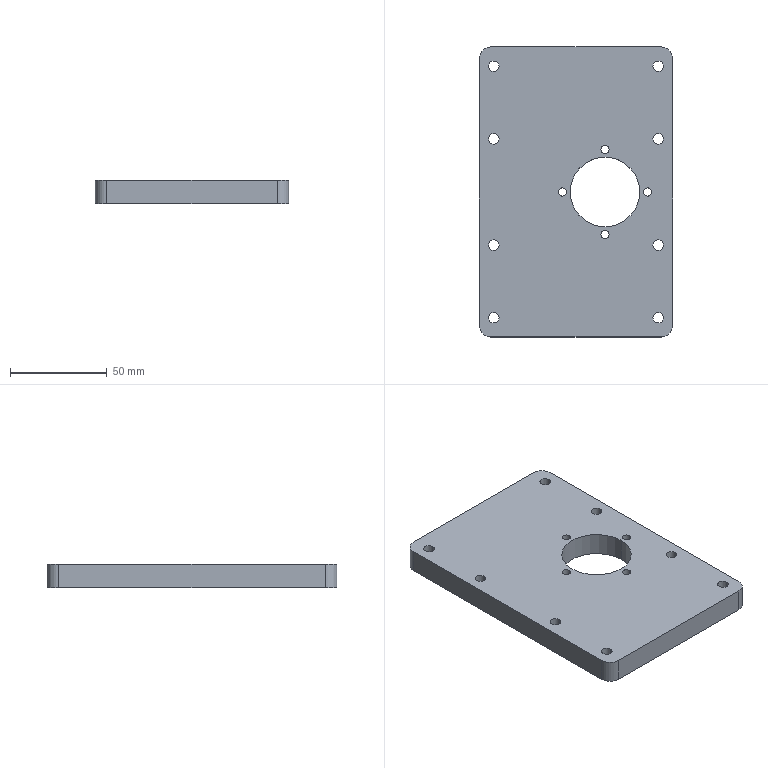Part | STEP file | QA-FC05 | 1 solid | 60 faces | box 100 x 150 x 12 mm | volume 162249 mm3 | cylinder 46 | plane 14 | commonest cylinder face diameters 5.5 x16 4.2 x8 9.5 x8 10 x8 12 x4 36 x2